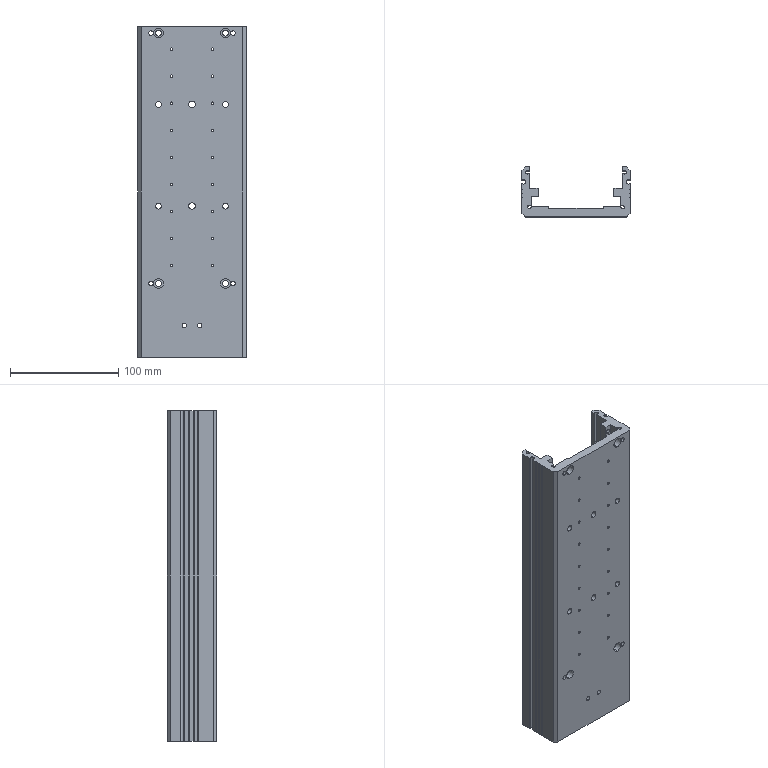Part | SolidWorks | features HoleWzd 8, ICE 3, 3DProfileFeature 1, Extrusion 1, LPattern 1, MirrorPattern 1 | 1 solid | 275 faces | box 100 x 46 x 306 mm | volume 422449 mm3 | cylinder 145 | plane 100 | spline 18 | cone 12 | commonest cylinder face diameters 2.5 x40 0.6 x22 4.2 x20 5.5 x16 3.3 x12 11 x12